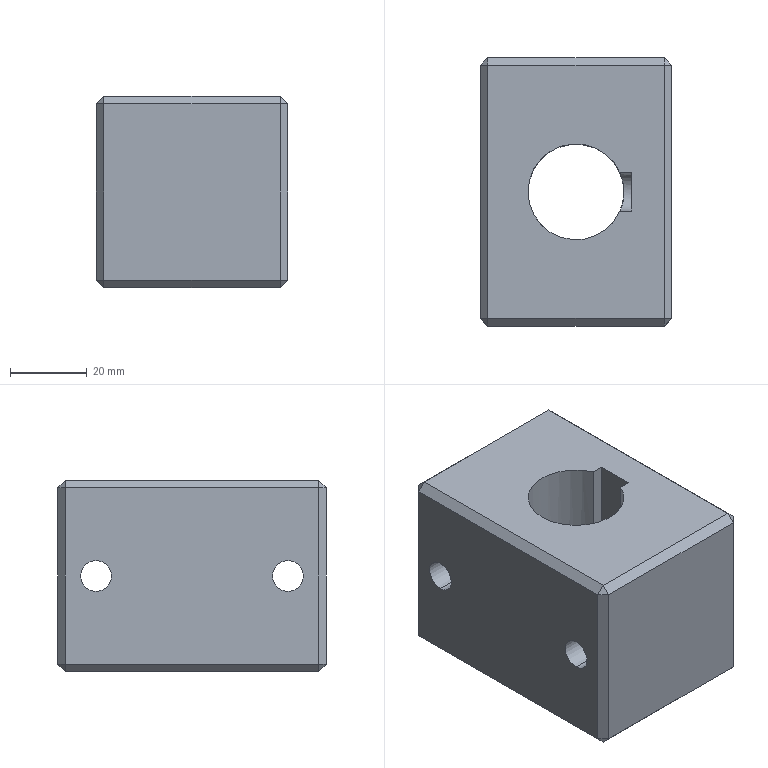Part | SolidWorks | features ICE 3, Chamfer 1, Extrusion 1, MirrorPattern 1 | 1 solid | 38 faces | box 50 x 70 x 50 mm | volume 143509 mm3 | plane 31 | cylinder 7 | commonest cylinder face diameters 8 x4 25 x2 10 x1
STEP:
#1=CARTESIAN_POINT('',(-25.,-25.,21.));
#2=VERTEX_POINT('',#1);
#3=CARTESIAN_POINT('',(-25.,-25.,29.));
#4=VERTEX_POINT('',#3);
#5=CARTESIAN_POINT('',(-25.,-25.,25.));
#6=DIRECTION('',(-1.,0.,0.));
#7=DIRECTION('',(0.,0.,-1.));
#8=AXIS2_PLACEMENT_3D('',#5,#6,#7);
#9=CIRCLE('',#8,4.);
#10=EDGE_CURVE('',#2,#4,#9,.T.);
#11=ORIENTED_EDGE('',*,*,#10,.T.);
#12=CARTESIAN_POINT('',(25.,-25.,29.));
#13=VERTEX_POINT('',#12);
#14=CARTESIAN_POINT('',(-33.,-25.,29.));
#15=DIRECTION('',(1.,0.,0.));
#16=VECTOR('',#15,1000.);
#17=LINE('',#14,#16);
#18=EDGE_CURVE('',#4,#13,#17,.T.);
#19=ORIENTED_EDGE('',*,*,#18,.T.);
#20=CARTESIAN_POINT('',(25.,-25.,21.));
#21=VERTEX_POINT('',#20);
#22=CARTESIAN_POINT('',(25.,-25.,25.));
#23=DIRECTION('',(-1.,0.,0.));
#24=DIRECTION('',(0.,0.,-1.));
#25=AXIS2_PLACEMENT_3D('',#22,#23,#24);
#26=CIRCLE('',#25,4.);
#27=EDGE_CURVE('',#21,#13,#26,.T.);
#28=ORIENTED_EDGE('',*,*,#27,.F.);
#29=CARTESIAN_POINT('',(-33.,-25.,21.));
#30=DIRECTION('',(1.,0.,0.));
#31=VECTOR('',#30,1000.);
#32=LINE('',#29,#31);
#33=EDGE_CURVE('',#2,#21,#32,.T.);
#34=ORIENTED_EDGE('',*,*,#33,.F.);
#35=EDGE_LOOP('',(#11,#19,#28,#34));
#36=FACE_OUTER_BOUND('',#35,.T.);
#37=CARTESIAN_POINT('',(-33.,-25.,25.));
#38=DIRECTION('',(1.,0.,0.));
#39=DIRECTION('',(0.,0.,-1.));
#40=AXIS2_PLACEMENT_3D('',#37,#38,#39);
#41=CYLINDRICAL_SURFACE('',#40,4.);
#42=ADVANCED_FACE('',(#36),#41,.F.);
#43=CARTESIAN_POINT('',(-25.,25.,29.));
#44=VERTEX_POINT('',#43);
#45=CARTESIAN_POINT('',(-25.,25.,21.));
#46=VERTEX_POINT('',#45);
#47=CARTESIAN_POINT('',(-25.,25.,25.));
#48=DIRECTION('',(1.,0.,0.));
#49=DIRECTION('',(0.,0.,-1.));
#50=AXIS2_PLACEMENT_3D('',#47,#48,#49);
#51=CIRCLE('',#50,4.);
#52=EDGE_CURVE('',#44,#46,#51,.T.);
#53=ORIENTED_EDGE('',*,*,#52,.F.);
#54=CARTESIAN_POINT('',(25.,25.,29.));
#55=VERTEX_POINT('',#54);
#56=CARTESIAN_POINT('',(-33.,25.,29.));
#57=DIRECTION('',(1.,0.,0.));
#58=VECTOR('',#57,1000.);
#59=LINE('',#56,#58);
#60=EDGE_CURVE('',#44,#55,#59,.T.);
#61=ORIENTED_EDGE('',*,*,#60,.T.);
#62=CARTESIAN_POINT('',(25.,25.,21.));
#63=VERTEX_POINT('',#62);
#64=CARTESIAN_POINT('',(25.,25.,25.));
#65=DIRECTION('',(1.,0.,0.));
#66=DIRECTION('',(0.,0.,-1.));
#67=AXIS2_PLACEMENT_3D('',#64,#65,#66);
#68=CIRCLE('',#67,4.);
#69=EDGE_CURVE('',#55,#63,#68,.T.);
#70=ORIENTED_EDGE('',*,*,#69,.T.);
#71=CARTESIAN_POINT('',(-33.,25.,21.));
#72=DIRECTION('',(1.,0.,0.));
#73=VECTOR('',#72,1000.);
#74=LINE('',#71,#73);
#75=EDGE_CURVE('',#46,#63,#74,.T.);
#76=ORIENTED_EDGE('',*,*,#75,.F.);
#77=EDGE_LOOP('',(#53,#61,#70,#76));
#78=FACE_OUTER_BOUND('',#77,.T.);
#79=CARTESIAN_POINT('',(-33.,25.,25.));
#80=DIRECTION('',(1.,0.,0.));
#81=DIRECTION('',(0.,0.,-1.));
#82=AXIS2_PLACEMENT_3D('',#79,#80,#81);
#83=CYLINDRICAL_SURFACE('',#82,4.);
#84=ADVANCED_FACE('',(#78),#83,.F.);
#85=CARTESIAN_POINT('',(-12.5,0.,0.));
#86=VERTEX_POINT('',#85);
#87=CARTESIAN_POINT('',(12.5,0.,0.));
#88=VERTEX_POINT('',#87);
#89=CARTESIAN_POINT('',(0.,0.,0.));
#90=DIRECTION('',(0.,0.,1.));
#91=DIRECTION('',(1.,0.,0.));
#92=AXIS2_PLACEMENT_3D('',#89,#90,#91);
#93=CIRCLE('',#92,12.5);
#94=EDGE_CURVE('',#86,#88,#93,.T.);
#95=ORIENTED_EDGE('',*,*,#94,.F.);
#96=CARTESIAN_POINT('',(-12.5,0.,50.));
#97=VERTEX_POINT('',#96);
#98=CARTESIAN_POINT('',(-12.5,0.,0.));
#99=DIRECTION('',(0.,0.,1.));
#100=VECTOR('',#99,1000.);
#101=LINE('',#98,#100);
#102=EDGE_CURVE('',#86,#97,#101,.T.);
#103=ORIENTED_EDGE('',*,*,#102,.T.);
#104=CARTESIAN_POINT('',(11.5,-4.899,50.));
#105=VERTEX_POINT('',#104);
#106=CARTESIAN_POINT('',(0.,0.,50.));
#107=DIRECTION('',(0.,0.,1.));
#108=DIRECTION('',(1.,0.,0.));
#109=AXIS2_PLACEMENT_3D('',#106,#107,#108);
#110=CIRCLE('',#109,12.5);
#111=EDGE_CURVE('',#97,#105,#110,.T.);
#112=ORIENTED_EDGE('',*,*,#111,.T.);
#113=CARTESIAN_POINT('',(11.5,-4.899,27.));
#114=VERTEX_POINT('',#113);
#115=CARTESIAN_POINT('',(11.5,-4.899,0.));
#116=DIRECTION('',(0.,0.,1.));
#117=VECTOR('',#116,1000.);
#118=LINE('',#115,#117);
#119=EDGE_CURVE('',#114,#105,#118,.T.);
#120=ORIENTED_EDGE('',*,*,#119,.F.);
#121=CARTESIAN_POINT('',(12.5,0.,23.));
#122=VERTEX_POINT('',#121);
#123=CARTESIAN_POINT('',(12.5,0.,23.));
#124=CARTESIAN_POINT('',(12.5,-0.2904,23.));
#125=CARTESIAN_POINT('',(12.49,-0.5768,23.025));
#126=CARTESIAN_POINT('',(12.451,-1.142,23.124));
#127=CARTESIAN_POINT('',(12.422,-1.423,23.198));
#128=CARTESIAN_POINT('',(12.348,-1.963,23.393));
#129=CARTESIAN_POINT('',(12.304,-2.222,23.512));
#130=CARTESIAN_POINT('',(12.204,-2.716,23.792));
#131=CARTESIAN_POINT('',(12.148,-2.953,23.955));
#132=CARTESIAN_POINT('',(12.034,-3.39,24.314));
#133=CARTESIAN_POINT('',(11.974,-3.592,24.51));
#134=CARTESIAN_POINT('',(11.857,-3.962,24.937));
#135=CARTESIAN_POINT('',(11.799,-4.131,25.169));
#136=CARTESIAN_POINT('',(11.692,-4.424,25.653));
#137=CARTESIAN_POINT('',(11.643,-4.549,25.906));
#138=CARTESIAN_POINT('',(11.56,-4.758,26.437));
#139=CARTESIAN_POINT('',(11.525,-4.841,26.715));
#140=CARTESIAN_POINT('',(11.5,-4.899,27.));
#141=B_SPLINE_CURVE_WITH_KNOTS('',3,(#123,#124,#125,#126,#127,#128,#129,#130,#131,#132,#133,#134,#135,#136,#137,#138,#139,#140),.UNSPECIFIED.,.F.,.F.,(4,2,2,2,2,2,2,2,4),(0.006896,0.007757,0.008619,0.00948,0.01034,0.0112,0.01206,0.01292,0.01379),.UNSPECIFIED.);
#142=EDGE_CURVE('',#122,#114,#141,.T.);
#143=ORIENTED_EDGE('',*,*,#142,.F.);
#144=CARTESIAN_POINT('',(12.5,0.,0.));
#145=DIRECTION('',(0.,0.,1.));
#146=VECTOR('',#145,1000.);
#147=LINE('',#144,#146);
#148=EDGE_CURVE('',#88,#122,#147,.T.);
#149=ORIENTED_EDGE('',*,*,#148,.F.);
#150=EDGE_LOOP('',(#95,#103,#112,#120,#143,#149));
#151=FACE_OUTER_BOUND('',#150,.T.);
#152=CARTESIAN_POINT('',(0.,0.,0.));
#153=DIRECTION('',(0.,0.,1.));
#154=DIRECTION('',(1.,0.,0.));
#155=AXIS2_PLACEMENT_3D('',#152,#153,#154);
#156=CYLINDRICAL_SURFACE('',#155,12.5);
#157=ADVANCED_FACE('',(#151),#156,.F.);
#158=ORIENTED_EDGE('',*,*,#102,.F.);
#159=CARTESIAN_POINT('',(0.,0.,0.));
#160=DIRECTION('',(0.,0.,1.));
#161=DIRECTION('',(1.,0.,0.));
#162=AXIS2_PLACEMENT_3D('',#159,#160,#161);
#163=CIRCLE('',#162,12.5);
#164=EDGE_CURVE('',#88,#86,#163,.T.);
#165=ORIENTED_EDGE('',*,*,#164,.F.);
#166=ORIENTED_EDGE('',*,*,#148,.T.);
#167=CARTESIAN_POINT('',(11.5,4.899,27.));
#168=VERTEX_POINT('',#167);
#169=CARTESIAN_POINT('',(11.5,4.899,27.));
#170=CARTESIAN_POINT('',(11.55,4.783,26.43));
#171=CARTESIAN_POINT('',(11.638,4.574,25.9));
#172=CARTESIAN_POINT('',(11.799,4.129,25.166));
#173=CARTESIAN_POINT('',(11.857,3.963,24.938));
#174=CARTESIAN_POINT('',(11.974,3.594,24.512));
#175=CARTESIAN_POINT('',(12.034,3.39,24.314));
#176=CARTESIAN_POINT('',(12.149,2.949,23.953));
#177=CARTESIAN_POINT('',(12.204,2.716,23.793));
#178=CARTESIAN_POINT('',(12.303,2.224,23.513));
#179=CARTESIAN_POINT('',(12.348,1.964,23.393));
#180=CARTESIAN_POINT('',(12.422,1.421,23.198));
#181=CARTESIAN_POINT('',(12.451,1.144,23.124));
#182=CARTESIAN_POINT('',(12.49,0.5802,23.026));
#183=CARTESIAN_POINT('',(12.5,0.2907,23.));
#184=CARTESIAN_POINT('',(12.5,0.,23.));
#185=B_SPLINE_CURVE_WITH_KNOTS('',3,(#169,#170,#171,#172,#173,#174,#175,#176,#177,#178,#179,#180,#181,#182,#183,#184),.UNSPECIFIED.,.F.,.F.,(4,2,2,2,2,2,2,4),(0.,0.001724,0.002586,0.003448,0.00431,0.005172,0.006034,0.006896),.UNSPECIFIED.);
#186=EDGE_CURVE('',#168,#122,#185,.T.);
#187=ORIENTED_EDGE('',*,*,#186,.F.);
#188=CARTESIAN_POINT('',(11.5,4.899,50.));
#189=VERTEX_POINT('',#188);
#190=CARTESIAN_POINT('',(11.5,4.899,0.));
#191=DIRECTION('',(0.,0.,-1.));
#192=VECTOR('',#191,1000.);
#193=LINE('',#190,#192);
#194=EDGE_CURVE('',#189,#168,#193,.T.);
#195=ORIENTED_EDGE('',*,*,#194,.F.);
#196=CARTESIAN_POINT('',(0.,0.,50.));
#197=DIRECTION('',(0.,0.,1.));
#198=DIRECTION('',(1.,0.,0.));
#199=AXIS2_PLACEMENT_3D('',#196,#197,#198);
#200=CIRCLE('',#199,12.5);
#201=EDGE_CURVE('',#189,#97,#200,.T.);
#202=ORIENTED_EDGE('',*,*,#201,.T.);
#203=EDGE_LOOP('',(#158,#165,#166,#187,#195,#202));
#204=FACE_OUTER_BOUND('',#203,.T.);
#205=CARTESIAN_POINT('',(0.,0.,0.));
#206=DIRECTION('',(0.,0.,1.));
#207=DIRECTION('',(1.,0.,0.));
#208=AXIS2_PLACEMENT_3D('',#205,#206,#207);
#209=CYLINDRICAL_SURFACE('',#208,12.5);
#210=ADVANCED_FACE('',(#204),#209,.F.);
#211=CARTESIAN_POINT('',(25.,-33.,48.));
#212=VERTEX_POINT('',#211);
#213=CARTESIAN_POINT('',(25.,-33.,2.));
#214=VERTEX_POINT('',#213);
#215=CARTESIAN_POINT('',(25.,-33.,50.));
#216=DIRECTION('',(0.,0.,-1.));
#217=VECTOR('',#216,1000.);
#218=LINE('',#215,#217);
#219=EDGE_CURVE('',#212,#214,#218,.T.);
#220=ORIENTED_EDGE('',*,*,#219,.T.);
#221=CARTESIAN_POINT('',(25.,33.,2.));
#222=VERTEX_POINT('',#221);
#223=CARTESIAN_POINT('',(25.,35.,2.));
#224=DIRECTION('',(0.,1.,0.));
#225=VECTOR('',#224,1000.);
#226=LINE('',#223,#225);
#227=EDGE_CURVE('',#214,#222,#226,.T.);
#228=ORIENTED_EDGE('',*,*,#227,.T.);
#229=CARTESIAN_POINT('',(25.,33.,48.));
#230=VERTEX_POINT('',#229);
#231=CARTESIAN_POINT('',(25.,33.,50.));
#232=DIRECTION('',(0.,0.,1.));
#233=VECTOR('',#232,1000.);
#234=LINE('',#231,#233);
#235=EDGE_CURVE('',#222,#230,#234,.T.);
#236=ORIENTED_EDGE('',*,*,#235,.T.);
#237=CARTESIAN_POINT('',(25.,-35.,48.));
#238=DIRECTION('',(0.,-1.,0.));
#239=VECTOR('',#238,1000.);
#240=LINE('',#237,#239);
#241=EDGE_CURVE('',#230,#212,#240,.T.);
#242=ORIENTED_EDGE('',*,*,#241,.T.);
#243=EDGE_LOOP('',(#220,#228,#236,#242));
#244=FACE_OUTER_BOUND('',#243,.T.);
#245=ORIENTED_EDGE('',*,*,#27,.T.);
#246=CARTESIAN_POINT('',(25.,-25.,25.));
#247=DIRECTION('',(-1.,0.,0.));
#248=DIRECTION('',(0.,0.,-1.));
#249=AXIS2_PLACEMENT_3D('',#246,#247,#248);
#250=CIRCLE('',#249,4.);
#251=EDGE_CURVE('',#13,#21,#250,.T.);
#252=ORIENTED_EDGE('',*,*,#251,.T.);
#253=EDGE_LOOP('',(#245,#252));
#254=FACE_BOUND('',#253,.T.);
#255=CARTESIAN_POINT('',(25.,25.,25.));
#256=DIRECTION('',(1.,0.,0.));
#257=DIRECTION('',(0.,0.,-1.));
#258=AXIS2_PLACEMENT_3D('',#255,#256,#257);
#259=CIRCLE('',#258,4.);
#260=EDGE_CURVE('',#63,#55,#259,.T.);
#261=ORIENTED_EDGE('',*,*,#260,.F.);
#262=ORIENTED_EDGE('',*,*,#69,.F.);
#263=EDGE_LOOP('',(#261,#262));
#264=FACE_BOUND('',#263,.T.);
#265=CARTESIAN_POINT('',(25.,-35.,50.));
#266=DIRECTION('',(-1.,0.,0.));
#267=DIRECTION('',(0.,0.,1.));
#268=AXIS2_PLACEMENT_3D('',#265,#266,#267);
#269=PLANE('',#268);
#270=ADVANCED_FACE('',(#244,#254,#264),#269,.F.);
#271=CARTESIAN_POINT('',(23.,35.,48.));
#272=VERTEX_POINT('',#271);
#273=CARTESIAN_POINT('',(23.,35.,2.));
#274=VERTEX_POINT('',#273);
#275=CARTESIAN_POINT('',(23.,35.,50.));
#276=DIRECTION('',(0.,0.,-1.));
#277=VECTOR('',#276,1000.);
#278=LINE('',#275,#277);
#279=EDGE_CURVE('',#272,#274,#278,.T.);
#280=ORIENTED_EDGE('',*,*,#279,.T.);
#281=CARTESIAN_POINT('',(-23.,35.,2.));
#282=VERTEX_POINT('',#281);
#283=CARTESIAN_POINT('',(-25.,35.,2.));
#284=DIRECTION('',(-1.,0.,0.));
#285=VECTOR('',#284,1000.);
#286=LINE('',#283,#285);
#287=EDGE_CURVE('',#274,#282,#286,.T.);
#288=ORIENTED_EDGE('',*,*,#287,.T.);
#289=CARTESIAN_POINT('',(-23.,35.,48.));
#290=VERTEX_POINT('',#289);
#291=CARTESIAN_POINT('',(-23.,35.,50.));
#292=DIRECTION('',(0.,0.,1.));
#293=VECTOR('',#292,1000.);
#294=LINE('',#291,#293);
#295=EDGE_CURVE('',#282,#290,#294,.T.);
#296=ORIENTED_EDGE('',*,*,#295,.T.);
#297=CARTESIAN_POINT('',(-25.,35.,48.));
#298=DIRECTION('',(1.,0.,0.));
#299=VECTOR('',#298,1000.);
#300=LINE('',#297,#299);
#301=EDGE_CURVE('',#290,#272,#300,.T.);
#302=ORIENTED_EDGE('',*,*,#301,.T.);
#303=EDGE_LOOP('',(#280,#288,#296,#302));
#304=FACE_OUTER_BOUND('',#303,.T.);
#305=CARTESIAN_POINT('',(-25.,35.,50.));
#306=DIRECTION('',(0.,-1.,0.));
#307=DIRECTION('',(0.,0.,-1.));
#308=AXIS2_PLACEMENT_3D('',#305,#306,#307);
#309=PLANE('',#308);
#310=ADVANCED_FACE('',(#304),#309,.F.);
#311=CARTESIAN_POINT('',(-25.,33.,48.));
#312=VERTEX_POINT('',#311);
#313=CARTESIAN_POINT('',(-25.,33.,2.));
#314=VERTEX_POINT('',#313);
#315=CARTESIAN_POINT('',(-25.,33.,50.));
#316=DIRECTION('',(0.,0.,-1.));
#317=VECTOR('',#316,1000.);
#318=LINE('',#315,#317);
#319=EDGE_CURVE('',#312,#314,#318,.T.);
#320=ORIENTED_EDGE('',*,*,#319,.T.);
#321=CARTESIAN_POINT('',(-25.,-33.,2.));
#322=VERTEX_POINT('',#321);
#323=CARTESIAN_POINT('',(-25.,-35.,2.));
#324=DIRECTION('',(0.,-1.,0.));
#325=VECTOR('',#324,1000.);
#326=LINE('',#323,#325);
#327=EDGE_CURVE('',#314,#322,#326,.T.);
#328=ORIENTED_EDGE('',*,*,#327,.T.);
#329=CARTESIAN_POINT('',(-25.,-33.,48.));
#330=VERTEX_POINT('',#329);
#331=CARTESIAN_POINT('',(-25.,-33.,50.));
#332=DIRECTION('',(0.,0.,1.));
#333=VECTOR('',#332,1000.);
#334=LINE('',#331,#333);
#335=EDGE_CURVE('',#322,#330,#334,.T.);
#336=ORIENTED_EDGE('',*,*,#335,.T.);
#337=CARTESIAN_POINT('',(-25.,-35.,48.));
#338=DIRECTION('',(0.,1.,0.));
#339=VECTOR('',#338,1000.);
#340=LINE('',#337,#339);
#341=EDGE_CURVE('',#330,#312,#340,.T.);
#342=ORIENTED_EDGE('',*,*,#341,.T.);
#343=EDGE_LOOP('',(#320,#328,#336,#342));
#344=FACE_OUTER_BOUND('',#343,.T.);
#345=ORIENTED_EDGE('',*,*,#10,.F.);
#346=CARTESIAN_POINT('',(-25.,-25.,25.));
#347=DIRECTION('',(-1.,0.,0.));
#348=DIRECTION('',(0.,0.,-1.));
#349=AXIS2_PLACEMENT_3D('',#346,#347,#348);
#350=CIRCLE('',#349,4.);
#351=EDGE_CURVE('',#4,#2,#350,.T.);
#352=ORIENTED_EDGE('',*,*,#351,.F.);
#353=EDGE_LOOP('',(#345,#352));
#354=FACE_BOUND('',#353,.T.);
#355=CARTESIAN_POINT('',(-25.,25.,25.));
#356=DIRECTION('',(1.,0.,0.));
#357=DIRECTION('',(0.,0.,-1.));
#358=AXIS2_PLACEMENT_3D('',#355,#356,#357);
#359=CIRCLE('',#358,4.);
#360=EDGE_CURVE('',#46,#44,#359,.T.);
#361=ORIENTED_EDGE('',*,*,#360,.T.);
#362=ORIENTED_EDGE('',*,*,#52,.T.);
#363=EDGE_LOOP('',(#361,#362));
#364=FACE_BOUND('',#363,.T.);
#365=CARTESIAN_POINT('',(-25.,-35.,50.));
#366=DIRECTION('',(1.,0.,0.));
#367=DIRECTION('',(0.,0.,-1.));
#368=AXIS2_PLACEMENT_3D('',#365,#366,#367);
#369=PLANE('',#368);
#370=ADVANCED_FACE('',(#344,#354,#364),#369,.F.);
#371=CARTESIAN_POINT('',(23.,-35.,48.));
#372=VERTEX_POINT('',#371);
#373=CARTESIAN_POINT('',(-23.,-35.,48.));
#374=VERTEX_POINT('',#373);
#375=CARTESIAN_POINT('',(-25.,-35.,48.));
#376=DIRECTION('',(-1.,0.,0.));
#377=VECTOR('',#376,1000.);
#378=LINE('',#375,#377);
#379=EDGE_CURVE('',#372,#374,#378,.T.);
#380=ORIENTED_EDGE('',*,*,#379,.T.);
#381=CARTESIAN_POINT('',(-23.,-35.,2.));
#382=VERTEX_POINT('',#381);
#383=CARTESIAN_POINT('',(-23.,-35.,50.));
#384=DIRECTION('',(0.,0.,-1.));
#385=VECTOR('',#384,1000.);
#386=LINE('',#383,#385);
#387=EDGE_CURVE('',#374,#382,#386,.T.);
#388=ORIENTED_EDGE('',*,*,#387,.T.);
#389=CARTESIAN_POINT('',(23.,-35.,2.));
#390=VERTEX_POINT('',#389);
#391=CARTESIAN_POINT('',(25.,-35.,2.));
#392=DIRECTION('',(1.,0.,0.));
#393=VECTOR('',#392,1000.);
#394=LINE('',#391,#393);
#395=EDGE_CURVE('',#382,#390,#394,.T.);
#396=ORIENTED_EDGE('',*,*,#395,.T.);
#397=CARTESIAN_POINT('',(23.,-35.,50.));
#398=DIRECTION('',(0.,0.,1.));
#399=VECTOR('',#398,1000.);
#400=LINE('',#397,#399);
#401=EDGE_CURVE('',#390,#372,#400,.T.);
#402=ORIENTED_EDGE('',*,*,#401,.T.);
#403=EDGE_LOOP('',(#380,#388,#396,#402));
#404=FACE_OUTER_BOUND('',#403,.T.);
#405=CARTESIAN_POINT('',(-25.,-35.,50.));
#406=DIRECTION('',(0.,1.,0.));
#407=DIRECTION('',(0.,0.,1.));
#408=AXIS2_PLACEMENT_3D('',#405,#406,#407);
#409=PLANE('',#408);
#410=ADVANCED_FACE('',(#404),#409,.F.);
#411=CARTESIAN_POINT('',(-23.,33.,50.));
#412=VERTEX_POINT('',#411);
#413=CARTESIAN_POINT('',(-23.,-33.,50.));
#414=VERTEX_POINT('',#413);
#415=CARTESIAN_POINT('',(-23.,0.,50.));
#416=DIRECTION('',(0.,-1.,0.));
#417=VECTOR('',#416,1000.);
#418=LINE('',#415,#417);
#419=EDGE_CURVE('',#412,#414,#418,.T.);
#420=ORIENTED_EDGE('',*,*,#419,.T.);
#421=CARTESIAN_POINT('',(23.,-33.,50.));
#422=VERTEX_POINT('',#421);
#423=CARTESIAN_POINT('',(0.,-33.,50.));
#424=DIRECTION('',(1.,0.,0.));
#425=VECTOR('',#424,1000.);
#426=LINE('',#423,#425);
#427=EDGE_CURVE('',#414,#422,#426,.T.);
#428=ORIENTED_EDGE('',*,*,#427,.T.);
#429=CARTESIAN_POINT('',(23.,33.,50.));
#430=VERTEX_POINT('',#429);
#431=CARTESIAN_POINT('',(23.,0.,50.));
#432=DIRECTION('',(0.,1.,0.));
#433=VECTOR('',#432,1000.);
#434=LINE('',#431,#433);
#435=EDGE_CURVE('',#422,#430,#434,.T.);
#436=ORIENTED_EDGE('',*,*,#435,.T.);
#437=CARTESIAN_POINT('',(0.,33.,50.));
#438=DIRECTION('',(-1.,0.,0.));
#439=VECTOR('',#438,1000.);
#440=LINE('',#437,#439);
#441=EDGE_CURVE('',#430,#412,#440,.T.);
#442=ORIENTED_EDGE('',*,*,#441,.T.);
#443=EDGE_LOOP('',(#420,#428,#436,#442));
#444=FACE_OUTER_BOUND('',#443,.T.);
#445=CARTESIAN_POINT('',(14.5,5.,50.));
#446=VERTEX_POINT('',#445);
#447=CARTESIAN_POINT('',(11.5,5.,50.));
#448=VERTEX_POINT('',#447);
#449=CARTESIAN_POINT('',(14.5,5.,50.));
#450=DIRECTION('',(-1.,0.,0.));
#451=VECTOR('',#450,1000.);
#452=LINE('',#449,#451);
#453=EDGE_CURVE('',#446,#448,#452,.T.);
#454=ORIENTED_EDGE('',*,*,#453,.F.);
#455=CARTESIAN_POINT('',(14.5,-5.,50.));
#456=VERTEX_POINT('',#455);
#457=CARTESIAN_POINT('',(14.5,0.,50.));
#458=DIRECTION('',(0.,-1.,0.));
#459=VECTOR('',#458,1000.);
#460=LINE('',#457,#459);
#461=EDGE_CURVE('',#446,#456,#460,.T.);
#462=ORIENTED_EDGE('',*,*,#461,.T.);
#463=CARTESIAN_POINT('',(11.5,-5.,50.));
#464=VERTEX_POINT('',#463);
#465=CARTESIAN_POINT('',(14.5,-5.,50.));
#466=DIRECTION('',(-1.,0.,0.));
#467=VECTOR('',#466,1000.);
#468=LINE('',#465,#467);
#469=EDGE_CURVE('',#456,#464,#468,.T.);
#470=ORIENTED_EDGE('',*,*,#469,.T.);
#471=CARTESIAN_POINT('',(11.5,0.,50.));
#472=DIRECTION('',(0.,-1.,0.));
#473=VECTOR('',#472,1000.);
#474=LINE('',#471,#473);
#475=EDGE_CURVE('',#105,#464,#474,.T.);
#476=ORIENTED_EDGE('',*,*,#475,.F.);
#477=ORIENTED_EDGE('',*,*,#111,.F.);
#478=ORIENTED_EDGE('',*,*,#201,.F.);
#479=CARTESIAN_POINT('',(11.5,0.,50.));
#480=DIRECTION('',(0.,-1.,0.));
#481=VECTOR('',#480,1000.);
#482=LINE('',#479,#481);
#483=EDGE_CURVE('',#448,#189,#482,.T.);
#484=ORIENTED_EDGE('',*,*,#483,.F.);
#485=EDGE_LOOP('',(#454,#462,#470,#476,#477,#478,#484));
#486=FACE_BOUND('',#485,.T.);
#487=CARTESIAN_POINT('',(0.,0.,50.));
#488=DIRECTION('',(0.,0.,-1.));
#489=DIRECTION('',(-1.,0.,0.));
#490=AXIS2_PLACEMENT_3D('',#487,#488,#489);
#491=PLANE('',#490);
#492=ADVANCED_FACE('',(#444,#486),#491,.F.);
#493=CARTESIAN_POINT('',(-23.,-33.,0.));
#494=VERTEX_POINT('',#493);
#495=CARTESIAN_POINT('',(-23.,33.,0.));
#496=VERTEX_POINT('',#495);
#497=CARTESIAN_POINT('',(-23.,35.,0.));
#498=DIRECTION('',(0.,1.,0.));
#499=VECTOR('',#498,1000.);
#500=LINE('',#497,#499);
#501=EDGE_CURVE('',#494,#496,#500,.T.);
#502=ORIENTED_EDGE('',*,*,#501,.T.);
#503=CARTESIAN_POINT('',(23.,33.,0.));
#504=VERTEX_POINT('',#503);
#505=CARTESIAN_POINT('',(25.,33.,0.));
#506=DIRECTION('',(1.,0.,0.));
#507=VECTOR('',#506,1000.);
#508=LINE('',#505,#507);
#509=EDGE_CURVE('',#496,#504,#508,.T.);
#510=ORIENTED_EDGE('',*,*,#509,.T.);
#511=CARTESIAN_POINT('',(23.,-33.,0.));
#512=VERTEX_POINT('',#511);
#513=CARTESIAN_POINT('',(23.,-35.,0.));
#514=DIRECTION('',(0.,-1.,0.));
#515=VECTOR('',#514,1000.);
#516=LINE('',#513,#515);
#517=EDGE_CURVE('',#504,#512,#516,.T.);
#518=ORIENTED_EDGE('',*,*,#517,.T.);
#519=CARTESIAN_POINT('',(-25.,-33.,0.));
#520=DIRECTION('',(-1.,0.,0.));
#521=VECTOR('',#520,1000.);
#522=LINE('',#519,#521);
#523=EDGE_CURVE('',#512,#494,#522,.T.);
#524=ORIENTED_EDGE('',*,*,#523,.T.);
#525=EDGE_LOOP('',(#502,#510,#518,#524));
#526=FACE_OUTER_BOUND('',#525,.T.);
#527=ORIENTED_EDGE('',*,*,#164,.T.);
#528=ORIENTED_EDGE('',*,*,#94,.T.);
#529=EDGE_LOOP('',(#527,#528));
#530=FACE_BOUND('',#529,.T.);
#531=CARTESIAN_POINT('',(0.,0.,0.));
#532=DIRECTION('',(0.,0.,-1.));
#533=DIRECTION('',(-1.,0.,0.));
#534=AXIS2_PLACEMENT_3D('',#531,#532,#533);
#535=PLANE('',#534);
#536=ADVANCED_FACE('',(#526,#530),#535,.T.);
#537=ORIENTED_EDGE('',*,*,#60,.F.);
#538=ORIENTED_EDGE('',*,*,#360,.F.);
#539=ORIENTED_EDGE('',*,*,#75,.T.);
#540=ORIENTED_EDGE('',*,*,#260,.T.);
#541=EDGE_LOOP('',(#537,#538,#539,#540));
#542=FACE_OUTER_BOUND('',#541,.T.);
#543=CARTESIAN_POINT('',(-33.,25.,25.));
#544=DIRECTION('',(1.,0.,0.));
#545=DIRECTION('',(0.,0.,-1.));
#546=AXIS2_PLACEMENT_3D('',#543,#544,#545);
#547=CYLINDRICAL_SURFACE('',#546,4.);
#548=ADVANCED_FACE('',(#542),#547,.F.);
#549=ORIENTED_EDGE('',*,*,#18,.F.);
#550=ORIENTED_EDGE('',*,*,#351,.T.);
#551=ORIENTED_EDGE('',*,*,#33,.T.);
#552=ORIENTED_EDGE('',*,*,#251,.F.);
#553=EDGE_LOOP('',(#549,#550,#551,#552));
#554=FACE_OUTER_BOUND('',#553,.T.);
#555=CARTESIAN_POINT('',(-33.,-25.,25.));
#556=DIRECTION('',(1.,0.,0.));
#557=DIRECTION('',(0.,0.,-1.));
#558=AXIS2_PLACEMENT_3D('',#555,#556,#557);
#559=CYLINDRICAL_SURFACE('',#558,4.);
#560=ADVANCED_FACE('',(#554),#559,.F.);
#561=CARTESIAN_POINT('',(23.,-33.,50.));
#562=DIRECTION('',(0.,-0.7071,-0.7071));
#563=VECTOR('',#562,1000.);
#564=LINE('',#561,#563);
#565=EDGE_CURVE('',#422,#372,#564,.T.);
#566=ORIENTED_EDGE('',*,*,#565,.F.);
#567=ORIENTED_EDGE('',*,*,#427,.F.);
#568=CARTESIAN_POINT('',(-23.,-34.,49.));
#569=DIRECTION('',(0.,0.7071,0.7071));
#570=VECTOR('',#569,1000.);
#571=LINE('',#568,#570);
#572=EDGE_CURVE('',#374,#414,#571,.T.);
#573=ORIENTED_EDGE('',*,*,#572,.F.);
#574=ORIENTED_EDGE('',*,*,#379,.F.);
#575=EDGE_LOOP('',(#566,#567,#573,#574));
#576=FACE_OUTER_BOUND('',#575,.T.);
#577=CARTESIAN_POINT('',(0.,-33.,50.));
#578=DIRECTION('',(0.,0.7071,-0.7071));
#579=DIRECTION('',(1.,0.,0.));
#580=AXIS2_PLACEMENT_3D('',#577,#578,#579);
#581=PLANE('',#580);
#582=ADVANCED_FACE('',(#576),#581,.F.);
#583=CARTESIAN_POINT('',(23.,-33.,50.));
#584=DIRECTION('',(0.7071,0.,-0.7071));
#585=VECTOR('',#584,1000.);
#586=LINE('',#583,#585);
#587=EDGE_CURVE('',#422,#212,#586,.T.);
#588=ORIENTED_EDGE('',*,*,#587,.F.);
#589=ORIENTED_EDGE('',*,*,#565,.T.);
#590=CARTESIAN_POINT('',(24.,-34.,48.));
#591=DIRECTION('',(-0.7071,-0.7071,0.));
#592=VECTOR('',#591,1000.);
#593=LINE('',#590,#592);
#594=EDGE_CURVE('',#212,#372,#593,.T.);
#595=ORIENTED_EDGE('',*,*,#594,.F.);
#596=EDGE_LOOP('',(#588,#589,#595));
#597=FACE_OUTER_BOUND('',#596,.T.);
#598=CARTESIAN_POINT('',(23.,-33.,50.));
#599=DIRECTION('',(0.5774,-0.5774,0.5774));
#600=DIRECTION('',(0.7071,0.7071,0.));
#601=AXIS2_PLACEMENT_3D('',#598,#599,#600);
#602=PLANE('',#601);
#603=ADVANCED_FACE('',(#597),#602,.T.);
#604=CARTESIAN_POINT('',(-25.,-33.,48.));
#605=DIRECTION('',(-0.7071,0.7071,0.));
#606=VECTOR('',#605,1000.);
#607=LINE('',#604,#606);
#608=EDGE_CURVE('',#374,#330,#607,.T.);
#609=ORIENTED_EDGE('',*,*,#608,.F.);
#610=ORIENTED_EDGE('',*,*,#572,.T.);
#611=CARTESIAN_POINT('',(-25.,-33.,48.));
#612=DIRECTION('',(0.7071,0.,0.7071));
#613=VECTOR('',#612,1000.);
#614=LINE('',#611,#613);
#615=EDGE_CURVE('',#330,#414,#614,.T.);
#616=ORIENTED_EDGE('',*,*,#615,.F.);
#617=EDGE_LOOP('',(#609,#610,#616));
#618=FACE_OUTER_BOUND('',#617,.T.);
#619=CARTESIAN_POINT('',(-25.,-33.,48.));
#620=DIRECTION('',(-0.5774,-0.5774,0.5774));
#621=DIRECTION('',(0.7071,-0.7071,0.));
#622=AXIS2_PLACEMENT_3D('',#619,#620,#621);
#623=PLANE('',#622);
#624=ADVANCED_FACE('',(#618),#623,.T.);
#625=ORIENTED_EDGE('',*,*,#594,.T.);
#626=ORIENTED_EDGE('',*,*,#401,.F.);
#627=CARTESIAN_POINT('',(24.,-34.,2.));
#628=DIRECTION('',(-0.7071,-0.7071,0.));
#629=VECTOR('',#628,1000.);
#630=LINE('',#627,#629);
#631=EDGE_CURVE('',#214,#390,#630,.T.);
#632=ORIENTED_EDGE('',*,*,#631,.F.);
#633=ORIENTED_EDGE('',*,*,#219,.F.);
#634=EDGE_LOOP('',(#625,#626,#632,#633));
#635=FACE_OUTER_BOUND('',#634,.T.);
#636=CARTESIAN_POINT('',(25.,-33.,50.));
#637=DIRECTION('',(-0.7071,0.7071,0.));
#638=DIRECTION('',(0.,0.,-1.));
#639=AXIS2_PLACEMENT_3D('',#636,#637,#638);
#640=PLANE('',#639);
#641=ADVANCED_FACE('',(#635),#640,.F.);
#642=ORIENTED_EDGE('',*,*,#587,.T.);
#643=ORIENTED_EDGE('',*,*,#241,.F.);
#644=CARTESIAN_POINT('',(23.,33.,50.));
#645=DIRECTION('',(0.7071,0.,-0.7071));
#646=VECTOR('',#645,1000.);
#647=LINE('',#644,#646);
#648=EDGE_CURVE('',#430,#230,#647,.T.);
#649=ORIENTED_EDGE('',*,*,#648,.F.);
#650=ORIENTED_EDGE('',*,*,#435,.F.);
#651=EDGE_LOOP('',(#642,#643,#649,#650));
#652=FACE_OUTER_BOUND('',#651,.T.);
#653=CARTESIAN_POINT('',(23.,0.,50.));
#654=DIRECTION('',(-0.7071,0.,-0.7071));
#655=DIRECTION('',(0.,1.,0.));
#656=AXIS2_PLACEMENT_3D('',#653,#654,#655);
#657=PLANE('',#656);
#658=ADVANCED_FACE('',(#652),#657,.F.);
#659=CARTESIAN_POINT('',(-23.,34.,49.));
#660=DIRECTION('',(0.,0.7071,-0.7071));
#661=VECTOR('',#660,1000.);
#662=LINE('',#659,#661);
#663=EDGE_CURVE('',#412,#290,#662,.T.);
#664=ORIENTED_EDGE('',*,*,#663,.F.);
#665=ORIENTED_EDGE('',*,*,#441,.F.);
#666=CARTESIAN_POINT('',(23.,33.,50.));
#667=DIRECTION('',(0.,-0.7071,0.7071));
#668=VECTOR('',#667,1000.);
#669=LINE('',#666,#668);
#670=EDGE_CURVE('',#272,#430,#669,.T.);
#671=ORIENTED_EDGE('',*,*,#670,.F.);
#672=ORIENTED_EDGE('',*,*,#301,.F.);
#673=EDGE_LOOP('',(#664,#665,#671,#672));
#674=FACE_OUTER_BOUND('',#673,.T.);
#675=CARTESIAN_POINT('',(0.,33.,50.));
#676=DIRECTION('',(0.,-0.7071,-0.7071));
#677=DIRECTION('',(-1.,0.,0.));
#678=AXIS2_PLACEMENT_3D('',#675,#676,#677);
#679=PLANE('',#678);
#680=ADVANCED_FACE('',(#674),#679,.F.);
#681=ORIENTED_EDGE('',*,*,#615,.T.);
#682=ORIENTED_EDGE('',*,*,#419,.F.);
#683=CARTESIAN_POINT('',(-25.,33.,48.));
#684=DIRECTION('',(0.7071,0.,0.7071));
#685=VECTOR('',#684,1000.);
#686=LINE('',#683,#685);
#687=EDGE_CURVE('',#312,#412,#686,.T.);
#688=ORIENTED_EDGE('',*,*,#687,.F.);
#689=ORIENTED_EDGE('',*,*,#341,.F.);
#690=EDGE_LOOP('',(#681,#682,#688,#689));
#691=FACE_OUTER_BOUND('',#690,.T.);
#692=CARTESIAN_POINT('',(-23.,0.,50.));
#693=DIRECTION('',(0.7071,0.,-0.7071));
#694=DIRECTION('',(0.,-1.,0.));
#695=AXIS2_PLACEMENT_3D('',#692,#693,#694);
#696=PLANE('',#695);
#697=ADVANCED_FACE('',(#691),#696,.F.);
#698=ORIENTED_EDGE('',*,*,#608,.T.);
#699=ORIENTED_EDGE('',*,*,#335,.F.);
#700=CARTESIAN_POINT('',(-25.,-33.,2.));
#701=DIRECTION('',(-0.7071,0.7071,0.));
#702=VECTOR('',#701,1000.);
#703=LINE('',#700,#702);
#704=EDGE_CURVE('',#382,#322,#703,.T.);
#705=ORIENTED_EDGE('',*,*,#704,.F.);
#706=ORIENTED_EDGE('',*,*,#387,.F.);
#707=EDGE_LOOP('',(#698,#699,#705,#706));
#708=FACE_OUTER_BOUND('',#707,.T.);
#709=CARTESIAN_POINT('',(-23.,-35.,50.));
#710=DIRECTION('',(0.7071,0.7071,0.));
#711=DIRECTION('',(0.,0.,-1.));
#712=AXIS2_PLACEMENT_3D('',#709,#710,#711);
#713=PLANE('',#712);
#714=ADVANCED_FACE('',(#708),#713,.F.);
#715=CARTESIAN_POINT('',(23.,-33.,0.));
#716=DIRECTION('',(0.,0.7071,-0.7071));
#717=VECTOR('',#716,1000.);
#718=LINE('',#715,#717);
#719=EDGE_CURVE('',#390,#512,#718,.T.);
#720=ORIENTED_EDGE('',*,*,#719,.F.);
#721=ORIENTED_EDGE('',*,*,#395,.F.);
#722=CARTESIAN_POINT('',(-23.,-34.,1.));
#723=DIRECTION('',(0.,-0.7071,0.7071));
#724=VECTOR('',#723,1000.);
#725=LINE('',#722,#724);
#726=EDGE_CURVE('',#494,#382,#725,.T.);
#727=ORIENTED_EDGE('',*,*,#726,.F.);
#728=ORIENTED_EDGE('',*,*,#523,.F.);
#729=EDGE_LOOP('',(#720,#721,#727,#728));
#730=FACE_OUTER_BOUND('',#729,.T.);
#731=CARTESIAN_POINT('',(-25.,-35.,2.));
#732=DIRECTION('',(0.,-0.7071,-0.7071));
#733=DIRECTION('',(-1.,0.,0.));
#734=AXIS2_PLACEMENT_3D('',#731,#732,#733);
#735=PLANE('',#734);
#736=ADVANCED_FACE('',(#730),#735,.T.);
#737=ORIENTED_EDGE('',*,*,#631,.T.);
#738=ORIENTED_EDGE('',*,*,#719,.T.);
#739=CARTESIAN_POINT('',(23.,-33.,0.));
#740=DIRECTION('',(-0.7071,0.,-0.7071));
#741=VECTOR('',#740,1000.);
#742=LINE('',#739,#741);
#743=EDGE_CURVE('',#214,#512,#742,.T.);
#744=ORIENTED_EDGE('',*,*,#743,.F.);
#745=EDGE_LOOP('',(#737,#738,#744));
#746=FACE_OUTER_BOUND('',#745,.T.);
#747=CARTESIAN_POINT('',(23.,-33.,0.));
#748=DIRECTION('',(0.5774,-0.5774,-0.5774));
#749=DIRECTION('',(-0.7071,0.,-0.7071));
#750=AXIS2_PLACEMENT_3D('',#747,#748,#749);
#751=PLANE('',#750);
#752=ADVANCED_FACE('',(#746),#751,.T.);
#753=ORIENTED_EDGE('',*,*,#670,.T.);
#754=ORIENTED_EDGE('',*,*,#648,.T.);
#755=CARTESIAN_POINT('',(24.,34.,48.));
#756=DIRECTION('',(0.7071,-0.7071,0.));
#757=VECTOR('',#756,1000.);
#758=LINE('',#755,#757);
#759=EDGE_CURVE('',#272,#230,#758,.T.);
#760=ORIENTED_EDGE('',*,*,#759,.F.);
#761=EDGE_LOOP('',(#753,#754,#760));
#762=FACE_OUTER_BOUND('',#761,.T.);
#763=CARTESIAN_POINT('',(23.,33.,50.));
#764=DIRECTION('',(0.5774,0.5774,0.5774));
#765=DIRECTION('',(0.7071,0.,-0.7071));
#766=AXIS2_PLACEMENT_3D('',#763,#764,#765);
#767=PLANE('',#766);
#768=ADVANCED_FACE('',(#762),#767,.T.);
#769=ORIENTED_EDGE('',*,*,#687,.T.);
#770=ORIENTED_EDGE('',*,*,#663,.T.);
#771=CARTESIAN_POINT('',(-25.,33.,48.));
#772=DIRECTION('',(0.7071,0.7071,0.));
#773=VECTOR('',#772,1000.);
#774=LINE('',#771,#773);
#775=EDGE_CURVE('',#312,#290,#774,.T.);
#776=ORIENTED_EDGE('',*,*,#775,.F.);
#777=EDGE_LOOP('',(#769,#770,#776));
#778=FACE_OUTER_BOUND('',#777,.T.);
#779=CARTESIAN_POINT('',(-25.,33.,48.));
#780=DIRECTION('',(-0.5774,0.5774,0.5774));
#781=DIRECTION('',(0.7071,0.,0.7071));
#782=AXIS2_PLACEMENT_3D('',#779,#780,#781);
#783=PLANE('',#782);
#784=ADVANCED_FACE('',(#778),#783,.T.);
#785=ORIENTED_EDGE('',*,*,#726,.T.);
#786=ORIENTED_EDGE('',*,*,#704,.T.);
#787=CARTESIAN_POINT('',(-25.,-33.,2.));
#788=DIRECTION('',(-0.7071,0.,0.7071));
#789=VECTOR('',#788,1000.);
#790=LINE('',#787,#789);
#791=EDGE_CURVE('',#494,#322,#790,.T.);
#792=ORIENTED_EDGE('',*,*,#791,.F.);
#793=EDGE_LOOP('',(#785,#786,#792));
#794=FACE_OUTER_BOUND('',#793,.T.);
#795=CARTESIAN_POINT('',(-25.,-33.,2.));
#796=DIRECTION('',(-0.5774,-0.5774,-0.5774));
#797=DIRECTION('',(-0.7071,0.,0.7071));
#798=AXIS2_PLACEMENT_3D('',#795,#796,#797);
#799=PLANE('',#798);
#800=ADVANCED_FACE('',(#794),#799,.T.);
#801=ORIENTED_EDGE('',*,*,#743,.T.);
#802=ORIENTED_EDGE('',*,*,#517,.F.);
#803=CARTESIAN_POINT('',(23.,33.,0.));
#804=DIRECTION('',(-0.7071,0.,-0.7071));
#805=VECTOR('',#804,1000.);
#806=LINE('',#803,#805);
#807=EDGE_CURVE('',#222,#504,#806,.T.);
#808=ORIENTED_EDGE('',*,*,#807,.F.);
#809=ORIENTED_EDGE('',*,*,#227,.F.);
#810=EDGE_LOOP('',(#801,#802,#808,#809));
#811=FACE_OUTER_BOUND('',#810,.T.);
#812=CARTESIAN_POINT('',(25.,-35.,2.));
#813=DIRECTION('',(0.7071,0.,-0.7071));
#814=DIRECTION('',(0.,-1.,0.));
#815=AXIS2_PLACEMENT_3D('',#812,#813,#814);
#816=PLANE('',#815);
#817=ADVANCED_FACE('',(#811),#816,.T.);
#818=ORIENTED_EDGE('',*,*,#759,.T.);
#819=ORIENTED_EDGE('',*,*,#235,.F.);
#820=CARTESIAN_POINT('',(24.,34.,2.));
#821=DIRECTION('',(0.7071,-0.7071,0.));
#822=VECTOR('',#821,1000.);
#823=LINE('',#820,#822);
#824=EDGE_CURVE('',#274,#222,#823,.T.);
#825=ORIENTED_EDGE('',*,*,#824,.F.);
#826=ORIENTED_EDGE('',*,*,#279,.F.);
#827=EDGE_LOOP('',(#818,#819,#825,#826));
#828=FACE_OUTER_BOUND('',#827,.T.);
#829=CARTESIAN_POINT('',(23.,35.,50.));
#830=DIRECTION('',(-0.7071,-0.7071,0.));
#831=DIRECTION('',(0.,0.,-1.));
#832=AXIS2_PLACEMENT_3D('',#829,#830,#831);
#833=PLANE('',#832);
#834=ADVANCED_FACE('',(#828),#833,.F.);
#835=ORIENTED_EDGE('',*,*,#775,.T.);
#836=ORIENTED_EDGE('',*,*,#295,.F.);
#837=CARTESIAN_POINT('',(-23.,35.,2.));
#838=DIRECTION('',(0.7071,0.7071,0.));
#839=VECTOR('',#838,1000.);
#840=LINE('',#837,#839);
#841=EDGE_CURVE('',#314,#282,#840,.T.);
#842=ORIENTED_EDGE('',*,*,#841,.F.);
#843=ORIENTED_EDGE('',*,*,#319,.F.);
#844=EDGE_LOOP('',(#835,#836,#842,#843));
#845=FACE_OUTER_BOUND('',#844,.T.);
#846=CARTESIAN_POINT('',(-25.,33.,50.));
#847=DIRECTION('',(0.7071,-0.7071,0.));
#848=DIRECTION('',(0.,0.,-1.));
#849=AXIS2_PLACEMENT_3D('',#846,#847,#848);
#850=PLANE('',#849);
#851=ADVANCED_FACE('',(#845),#850,.F.);
#852=ORIENTED_EDGE('',*,*,#791,.T.);
#853=ORIENTED_EDGE('',*,*,#327,.F.);
#854=CARTESIAN_POINT('',(-24.,33.,1.));
#855=DIRECTION('',(-0.7071,0.,0.7071));
#856=VECTOR('',#855,1000.);
#857=LINE('',#854,#856);
#858=EDGE_CURVE('',#496,#314,#857,.T.);
#859=ORIENTED_EDGE('',*,*,#858,.F.);
#860=ORIENTED_EDGE('',*,*,#501,.F.);
#861=EDGE_LOOP('',(#852,#853,#859,#860));
#862=FACE_OUTER_BOUND('',#861,.T.);
#863=CARTESIAN_POINT('',(-25.,-35.,2.));
#864=DIRECTION('',(-0.7071,0.,-0.7071));
#865=DIRECTION('',(0.,1.,0.));
#866=AXIS2_PLACEMENT_3D('',#863,#864,#865);
#867=PLANE('',#866);
#868=ADVANCED_FACE('',(#862),#867,.T.);
#869=ORIENTED_EDGE('',*,*,#824,.T.);
#870=ORIENTED_EDGE('',*,*,#807,.T.);
#871=CARTESIAN_POINT('',(23.,33.,0.));
#872=DIRECTION('',(0.,-0.7071,-0.7071));
#873=VECTOR('',#872,1000.);
#874=LINE('',#871,#873);
#875=EDGE_CURVE('',#274,#504,#874,.T.);
#876=ORIENTED_EDGE('',*,*,#875,.F.);
#877=EDGE_LOOP('',(#869,#870,#876));
#878=FACE_OUTER_BOUND('',#877,.T.);
#879=CARTESIAN_POINT('',(23.,33.,0.));
#880=DIRECTION('',(0.5774,0.5774,-0.5774));
#881=DIRECTION('',(-0.7071,0.,-0.7071));
#882=AXIS2_PLACEMENT_3D('',#879,#880,#881);
#883=PLANE('',#882);
#884=ADVANCED_FACE('',(#878),#883,.T.);
#885=ORIENTED_EDGE('',*,*,#858,.T.);
#886=ORIENTED_EDGE('',*,*,#841,.T.);
#887=CARTESIAN_POINT('',(-23.,35.,2.));
#888=DIRECTION('',(0.,0.7071,0.7071));
#889=VECTOR('',#888,1000.);
#890=LINE('',#887,#889);
#891=EDGE_CURVE('',#496,#282,#890,.T.);
#892=ORIENTED_EDGE('',*,*,#891,.F.);
#893=EDGE_LOOP('',(#885,#886,#892));
#894=FACE_OUTER_BOUND('',#893,.T.);
#895=CARTESIAN_POINT('',(-23.,35.,2.));
#896=DIRECTION('',(-0.5774,0.5774,-0.5774));
#897=DIRECTION('',(-0.7071,0.,0.7071));
#898=AXIS2_PLACEMENT_3D('',#895,#896,#897);
#899=PLANE('',#898);
#900=ADVANCED_FACE('',(#894),#899,.T.);
#901=ORIENTED_EDGE('',*,*,#875,.T.);
#902=ORIENTED_EDGE('',*,*,#509,.F.);
#903=ORIENTED_EDGE('',*,*,#891,.T.);
#904=ORIENTED_EDGE('',*,*,#287,.F.);
#905=EDGE_LOOP('',(#901,#902,#903,#904));
#906=FACE_OUTER_BOUND('',#905,.T.);
#907=CARTESIAN_POINT('',(-25.,35.,2.));
#908=DIRECTION('',(0.,0.7071,-0.7071));
#909=DIRECTION('',(1.,0.,0.));
#910=AXIS2_PLACEMENT_3D('',#907,#908,#909);
#911=PLANE('',#910);
#912=ADVANCED_FACE('',(#906),#911,.T.);
#913=CARTESIAN_POINT('',(14.5,5.,28.));
#914=VERTEX_POINT('',#913);
#915=CARTESIAN_POINT('',(14.5,5.,50.));
#916=DIRECTION('',(0.,0.,1.));
#917=VECTOR('',#916,1000.);
#918=LINE('',#915,#917);
#919=EDGE_CURVE('',#914,#446,#918,.T.);
#920=ORIENTED_EDGE('',*,*,#919,.F.);
#921=CARTESIAN_POINT('',(14.5,-5.,28.));
#922=VERTEX_POINT('',#921);
#923=CARTESIAN_POINT('',(14.5,0.,28.));
#924=DIRECTION('',(1.,0.,0.));
#925=DIRECTION('',(0.,0.,-1.));
#926=AXIS2_PLACEMENT_3D('',#923,#924,#925);
#927=CIRCLE('',#926,5.);
#928=EDGE_CURVE('',#922,#914,#927,.T.);
#929=ORIENTED_EDGE('',*,*,#928,.F.);
#930=CARTESIAN_POINT('',(14.5,-5.,50.));
#931=DIRECTION('',(0.,0.,-1.));
#932=VECTOR('',#931,1000.);
#933=LINE('',#930,#932);
#934=EDGE_CURVE('',#456,#922,#933,.T.);
#935=ORIENTED_EDGE('',*,*,#934,.F.);
#936=ORIENTED_EDGE('',*,*,#461,.F.);
#937=EDGE_LOOP('',(#920,#929,#935,#936));
#938=FACE_OUTER_BOUND('',#937,.T.);
#939=CARTESIAN_POINT('',(14.5,0.,50.));
#940=DIRECTION('',(1.,0.,0.));
#941=DIRECTION('',(0.,0.,-1.));
#942=AXIS2_PLACEMENT_3D('',#939,#940,#941);
#943=PLANE('',#942);
#944=ADVANCED_FACE('',(#938),#943,.F.);
#945=ORIENTED_EDGE('',*,*,#186,.T.);
#946=ORIENTED_EDGE('',*,*,#142,.T.);
#947=CARTESIAN_POINT('',(11.5,-5.,28.));
#948=VERTEX_POINT('',#947);
#949=CARTESIAN_POINT('',(11.5,0.,28.));
#950=DIRECTION('',(1.,0.,0.));
#951=DIRECTION('',(0.,0.,-1.));
#952=AXIS2_PLACEMENT_3D('',#949,#950,#951);
#953=CIRCLE('',#952,5.);
#954=EDGE_CURVE('',#948,#114,#953,.T.);
#955=ORIENTED_EDGE('',*,*,#954,.F.);
#956=CARTESIAN_POINT('',(14.5,-5.,28.));
#957=DIRECTION('',(-1.,0.,0.));
#958=VECTOR('',#957,1000.);
#959=LINE('',#956,#958);
#960=EDGE_CURVE('',#922,#948,#959,.T.);
#961=ORIENTED_EDGE('',*,*,#960,.F.);
#962=ORIENTED_EDGE('',*,*,#928,.T.);
#963=CARTESIAN_POINT('',(11.5,5.,28.));
#964=VERTEX_POINT('',#963);
#965=CARTESIAN_POINT('',(14.5,5.,28.));
#966=DIRECTION('',(-1.,0.,0.));
#967=VECTOR('',#966,1000.);
#968=LINE('',#965,#967);
#969=EDGE_CURVE('',#914,#964,#968,.T.);
#970=ORIENTED_EDGE('',*,*,#969,.T.);
#971=CARTESIAN_POINT('',(11.5,0.,28.));
#972=DIRECTION('',(1.,0.,0.));
#973=DIRECTION('',(0.,0.,-1.));
#974=AXIS2_PLACEMENT_3D('',#971,#972,#973);
#975=CIRCLE('',#974,5.);
#976=EDGE_CURVE('',#168,#964,#975,.T.);
#977=ORIENTED_EDGE('',*,*,#976,.F.);
#978=EDGE_LOOP('',(#945,#946,#955,#961,#962,#970,#977));
#979=FACE_OUTER_BOUND('',#978,.T.);
#980=CARTESIAN_POINT('',(14.5,0.,28.));
#981=DIRECTION('',(-1.,0.,0.));
#982=DIRECTION('',(0.,0.,1.));
#983=AXIS2_PLACEMENT_3D('',#980,#981,#982);
#984=CYLINDRICAL_SURFACE('',#983,5.);
#985=ADVANCED_FACE('',(#979),#984,.F.);
#986=ORIENTED_EDGE('',*,*,#483,.T.);
#987=ORIENTED_EDGE('',*,*,#194,.T.);
#988=ORIENTED_EDGE('',*,*,#976,.T.);
#989=CARTESIAN_POINT('',(11.5,5.,50.));
#990=DIRECTION('',(0.,0.,1.));
#991=VECTOR('',#990,1000.);
#992=LINE('',#989,#991);
#993=EDGE_CURVE('',#964,#448,#992,.T.);
#994=ORIENTED_EDGE('',*,*,#993,.T.);
#995=EDGE_LOOP('',(#986,#987,#988,#994));
#996=FACE_OUTER_BOUND('',#995,.T.);
#997=CARTESIAN_POINT('',(11.5,0.,50.));
#998=DIRECTION('',(1.,0.,0.));
#999=DIRECTION('',(0.,0.,-1.));
#1000=AXIS2_PLACEMENT_3D('',#997,#998,#999);
#1001=PLANE('',#1000);
#1002=ADVANCED_FACE('',(#996),#1001,.T.);
#1003=ORIENTED_EDGE('',*,*,#475,.T.);
#1004=CARTESIAN_POINT('',(11.5,-5.,50.));
#1005=DIRECTION('',(0.,0.,-1.));
#1006=VECTOR('',#1005,1000.);
#1007=LINE('',#1004,#1006);
#1008=EDGE_CURVE('',#464,#948,#1007,.T.);
#1009=ORIENTED_EDGE('',*,*,#1008,.T.);
#1010=ORIENTED_EDGE('',*,*,#954,.T.);
#1011=ORIENTED_EDGE('',*,*,#119,.T.);
#1012=EDGE_LOOP('',(#1003,#1009,#1010,#1011));
#1013=FACE_OUTER_BOUND('',#1012,.T.);
#1014=CARTESIAN_POINT('',(11.5,0.,50.));
#1015=DIRECTION('',(1.,0.,0.));
#1016=DIRECTION('',(0.,0.,-1.));
#1017=AXIS2_PLACEMENT_3D('',#1014,#1015,#1016);
#1018=PLANE('',#1017);
#1019=ADVANCED_FACE('',(#1013),#1018,.T.);
#1020=ORIENTED_EDGE('',*,*,#1008,.F.);
#1021=ORIENTED_EDGE('',*,*,#469,.F.);
#1022=ORIENTED_EDGE('',*,*,#934,.T.);
#1023=ORIENTED_EDGE('',*,*,#960,.T.);
#1024=EDGE_LOOP('',(#1020,#1021,#1022,#1023));
#1025=FACE_OUTER_BOUND('',#1024,.T.);
#1026=CARTESIAN_POINT('',(14.5,-5.,50.));
#1027=DIRECTION('',(0.,1.,0.));
#1028=DIRECTION('',(0.,0.,1.));
#1029=AXIS2_PLACEMENT_3D('',#1026,#1027,#1028);
#1030=PLANE('',#1029);
#1031=ADVANCED_FACE('',(#1025),#1030,.T.);
#1032=ORIENTED_EDGE('',*,*,#993,.F.);
#1033=ORIENTED_EDGE('',*,*,#969,.F.);
#1034=ORIENTED_EDGE('',*,*,#919,.T.);
#1035=ORIENTED_EDGE('',*,*,#453,.T.);
#1036=EDGE_LOOP('',(#1032,#1033,#1034,#1035));
#1037=FACE_OUTER_BOUND('',#1036,.T.);
#1038=CARTESIAN_POINT('',(14.5,5.,50.));
#1039=DIRECTION('',(0.,-1.,0.));
#1040=DIRECTION('',(0.,0.,-1.));
#1041=AXIS2_PLACEMENT_3D('',#1038,#1039,#1040);
#1042=PLANE('',#1041);
#1043=ADVANCED_FACE('',(#1037),#1042,.T.);
#1044=CLOSED_SHELL('',(#42,#84,#157,#210,#270,#310,#370,#410,#492,#536,#548,#560,#582,#603,#624,#641,#658,#680,#697,#714,#736,#752,#768,#784,#800,#817,#834,#851,#868,#884,#900,#912,#944,#985,#1002,#1019,#1031,#1043));
#1045=MANIFOLD_SOLID_BREP('',#1044);
#1046=CARTESIAN_POINT('',(0.,0.,0.));
#1047=DIRECTION('',(0.,0.,1.));
#1048=DIRECTION('',(1.,0.,0.));
#1049=AXIS2_PLACEMENT_3D('',#1046,#1047,#1048);
#1050=(LENGTH_UNIT()NAMED_UNIT(*)SI_UNIT(.MILLI.,.METRE.));
#1051=UNCERTAINTY_MEASURE_WITH_UNIT(LENGTH_MEASURE(0.00001),#1050,'','');
#1052=(NAMED_UNIT(*)PLANE_ANGLE_UNIT()SI_UNIT($,.RADIAN.));
#1053=(NAMED_UNIT(*)SI_UNIT($,.STERADIAN.)SOLID_ANGLE_UNIT());
#1054=(GEOMETRIC_REPRESENTATION_CONTEXT(3)GLOBAL_UNCERTAINTY_ASSIGNED_CONTEXT((#1051))GLOBAL_UNIT_ASSIGNED_CONTEXT((#1050,#1052,#1053))REPRESENTATION_CONTEXT('',''));
#1055=ADVANCED_BREP_SHAPE_REPRESENTATION('',(#1045,#1049),#1054);